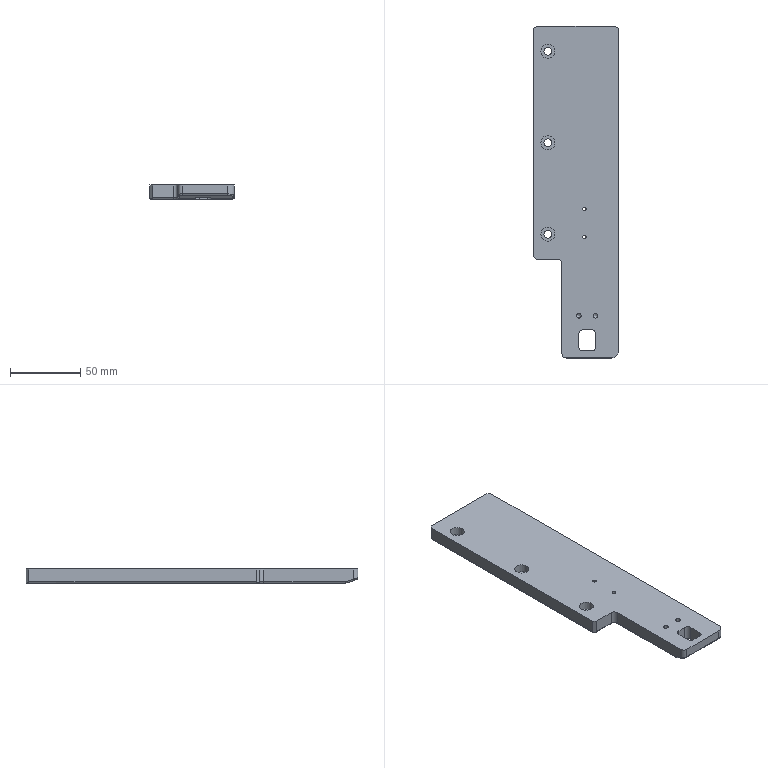NC program | NX | posted with a generic post | part box 60 x 236 x 10 mm
Lines 1177 to 2922 of 2922, first 1565 of 1740 lines:
(ZLEVEL_PROFILE_2 , TOOL : D4R0.5)
N2304 T17 M6
N2306 G54
N2308 G17 G0 G90 X-1.933 Y1.356 S9500 M3
N2310 G43 Z30. H17
N2312 Z1.488
N2314 G94 G1 Z-0.012 F3000.
N2316 X-1.63 Y0.83
N2318 G3 X-1.283 Y0.63 R0.4
N2320 G1 X0.698
N2322 X1.125 Y0.689
N2324 X164.875
N2326 G2 X166.689 Y-1.125 R1.915
N2328 G1 Y-17.
N2330 G3 X169. Y-19.311 R2.311
N2332 G1 X227.093
N2334 X227.441 Y-19.344
N2336 X229.095 Y-19.374
N2338 Y-19.313 Z-0.02
N2340 X229.094 Y-19.26 Z-0.028
N2342 X227.378 Y-19.24
N2344 X227.093 Y-19.21
N2346 X169.
N2348 G2 X166.79 Y-17. R2.21
N2350 G1 Y-1.191
N2352 G3 X164.809 Y0.79 R1.981
N2354 G1 X1.191
N2356 G2 X-1.267 Y0.741 R21.196
N2358 G1 X-1.234 Y0.83 Z-0.049
N2360 X0.863 Y0.842
N2362 X1.263 Y0.881
N2364 X164.752
N2366 G2 X166.881 Y-1.248 R2.129
N2368 G1 Y-17.
N2370 G3 X169. Y-19.119 R2.119
N2372 G1 X227.093
N2374 X227.378 Y-19.149
N2376 X229.092 Y-19.161
N2378 X229.089 Y-19.105 Z-0.063
N2380 X229.088 Y-19.063 Z-0.077
N2382 X227.232 Y-19.039
N2384 X227.093 Y-19.027
N2386 X169.
N2388 G2 X166.973 Y-17. R2.027
N2390 G1 Y-1.4
N2392 G3 X166.327 Y0.392 R2.646
N2394 X164.631 Y0.973 R2.773
N2396 G1 X1.546
N2398 G2 X-1.202 Y0.908 R23.914
N2400 G1 X-1.164 Y0.998 Z-0.11
N2402 G3 X1.546 Y1.064 R24.423
N2404 G1 X164.348
N2406 X164.631 Y1.063
N2408 X165.856 Y0.862
N2410 X166.009 Y0.8
N2412 G2 X166.917 Y-0.358 R1.468
N2414 G1 X167.064 Y-1.4
N2416 Y-17.
N2418 G3 X169. Y-18.936 R1.936
N2420 G1 X227.093
N2422 X227.254 Y-18.944
N2424 X227.378 Y-18.953
N2426 X227.661 Y-18.987
N2428 X229.087 Y-18.986
N2430 X229.086 Y-18.923 Z-0.13
N2432 Y-18.894 Z-0.15
N2434 X227.661 Y-18.896
N2436 X227.366 Y-18.863
N2438 X227.259 Y-18.858
N2440 X227.093 Y-18.847
N2442 X169.
N2444 G2 X167.153 Y-17. R1.847
N2446 G1 Y-1.681
N2448 X167.071 Y-0.473
N2450 G3 X165.738 Y1.034 R1.648
N2452 G1 X165.62 Y1.057
N2454 X164.569 Y1.15
N2456 X164.348 Y1.153
N2458 X1.546
N2460 X1.065 Y1.123
N2462 X-1.119 Y1.107
N2464 X-1.079 Y1.2 Z-0.195
N2466 G3 X1.546 Y1.24 R35.981
N2468 G1 X164.348
N2470 X165.536 Y1.173
N2472 X165.665 Y1.158
N2474 G2 X167.177 Y-0.455 R1.713
N2476 G1 X167.24 Y-1.681
N2478 Y-17.
N2480 G3 X169. Y-18.76 R1.76
N2482 G1 X227.093
N2484 G3 X229.084 Y-18.788 R19.848
N2486 G1 X229.085 Y-18.741 Z-0.221
N2488 Y-18.709 Z-0.247
N2490 X228.791 Y-18.697
N2492 X227.378 Y-18.703
N2494 X227.093 Y-18.676
N2496 X169.
N2498 G2 X167.324 Y-17. R1.676
N2500 G1 Y-1.547
N2502 X167.272 Y-0.402
N2504 G3 X165.609 Y1.264 R1.748
N2506 G1 X164.348 Y1.324
N2508 X1.547
N2510 G2 X0.774 Y1.287 R7.977
N2512 G1 X-1.035 Y1.288
N2514 X-0.987 Y1.376 Z-0.304
N2516 X1.263 Y1.381
N2518 X1.602 Y1.405
N2520 X164.398
N2522 X164.631 Y1.391
N2524 X165.657 Y1.35
N2526 G2 X167.356 Y-0.362 R1.77
N2528 G1 X167.39 Y-1.4
N2530 X167.405 Y-1.602
N2532 Y-17.
N2534 G3 X169. Y-18.595 R1.595
N2536 G1 X227.093
N2538 G3 X227.497 Y-18.618 R3.817
N2540 G1 X229.085 Y-18.628
N2542 X229.084 Y-18.592 Z-0.335
N2544 Y-18.556 Z-0.366
N2546 X227.661 Y-18.552
N2548 X227.519 Y-18.545
N2550 X227.292 Y-18.532
N2552 X227.093 Y-18.518
N2554 X169.
N2556 G2 X167.482 Y-17. R1.518
N2558 G1 Y-1.654
N2560 X167.466 Y-1.4
N2562 X167.441 Y-0.33
N2564 G3 X165.701 Y1.427 R1.799
N2566 G2 X164.346 Y1.482 R86.521
N2568 G1 X1.654
N2570 X1.546 Y1.474
N2572 X0.698 Y1.45
N2574 X-0.715 Y1.458
N2576 X-0.943 Y1.452
N2578 X-0.898 Y1.529 Z-0.434
N2580 X0.698 Y1.527
N2582 X1.546 Y1.548
N2584 X1.703 Y1.555
N2586 X164.297
N2588 X164.348 Y1.552
N2590 X165.757 Y1.504
N2592 G2 X167.518 Y-0.351 R1.825
N2594 G3 X167.555 Y-1.703 R15.073
N2596 G1 Y-17.
N2598 G3 X169. Y-18.445 R1.445
N2600 G1 X227.093
N2602 X227.286 Y-18.456
N2604 X227.481 Y-18.464
N2606 X227.661 Y-18.474
N2608 X228.509 Y-18.481
N2610 X229.083 Y-18.483
N2612 Y-18.442 Z-0.47
N2614 Y-18.412 Z-0.506
N2616 G2 X227.413 Y-18.393 R46.566
N2618 G1 X227.347 Y-18.39
N2620 X227.093 Y-18.377
N2622 X169.
N2624 G2 X167.623 Y-17. R1.377
N2626 G1 Y-1.747
N2628 G2 X167.591 Y-0.279 R21.059
N2630 G3 X165.762 Y1.577 R1.859
N2632 G2 X164.253 Y1.623 R51.61
N2634 G1 X1.747
N2636 X1.546 Y1.609
N2638 X0.698 Y1.594
N2640 X-0.715 Y1.598
N2642 X-0.85 Y1.594
N2644 X-0.798 Y1.66 Z-0.583
N2646 X-0.715 Y1.664
N2648 X0.971 Y1.66
N2650 G3 X1.791 Y1.687 R11.853
N2652 G1 X164.209
N2654 G3 X165.762 Y1.645 R86.835
N2656 G2 X167.321 Y0.842 R1.933
N2658 X167.659 Y-0.279 R1.92
N2660 G3 X167.687 Y-1.791 R14.568
N2662 G1 Y-17.
N2664 G3 X169. Y-18.313 R1.313
N2666 G1 X227.093
N2668 G3 X229.084 Y-18.34 R29.332
N2670 G1 X229.083 Y-18.306 Z-0.623
N2672 Y-18.273 Z-0.664
N2674 G2 X227.093 Y-18.255 R26.061
N2676 G1 X169.
N2678 G2 X167.745 Y-17. R1.255
N2680 G1 Y-1.828
N2682 G2 X167.72 Y-0.279 R18.813
N2684 G3 X167.406 Y0.842 R1.968
N2686 X165.762 Y1.71 R1.98
N2688 G2 X164.172 Y1.745 R28.102
N2690 G1 X1.828
N2692 G2 X1.263 Y1.718 R5.619
N2694 G1 X-0.747 Y1.721
N2696 X-0.697 Y1.774 Z-0.749
N2698 X1.263 Y1.77
N2700 G3 X1.864 Y1.798 R5.314
N2702 G1 X164.136
N2704 G3 X165.479 Y1.767 R16.419
N2706 G2 X166.234 Y1.707 R3.44
N2708 X167.773 Y-0.21 R1.898
N2710 G3 X167.798 Y-1.864 R19.045
N2712 G1 Y-17.
N2714 G3 X169. Y-18.202 R1.202
N2716 G1 X227.093
N2718 G3 X227.701 Y-18.217 R11.739
N2720 G1 X229.082
N2722 Y-18.196 Z-0.793
N2724 Y-18.172 Z-0.837
N2726 G2 X227.093 Y-18.155 R38.055
N2728 G1 X169.
N2730 G2 X167.845 Y-17. R1.155
N2732 G1 Y-1.895
N2734 G2 X167.819 Y-0.279 R20.129
N2736 G1 X167.815 Y-0.077
N2738 G3 X166.196 Y1.765 R1.895
N2740 X165.196 Y1.824 R5.764
N2742 G2 X164.105 Y1.845 R13.41
N2744 G1 X1.895
N2746 G2 X1.249 Y1.822 R8.509
N2748 G1 X-0.433 Y1.826
N2750 X-0.646 Y1.821
N2752 X-0.594 Y1.864 Z-0.928
N2754 X-0.433 Y1.866
N2756 X1.247 Y1.862
N2758 G3 X1.923 Y1.887 R8.855
N2760 G1 X164.077
N2762 G3 X165.196 Y1.864 R12.939
N2764 G2 X166.09 Y1.831 R9.187
N2766 X167.868 Y-0.096 R1.942
N2768 G1 X167.874 Y-1.681
N2770 X167.887 Y-1.923
N2772 Y-17.
N2774 G3 X169. Y-18.113 R1.113
N2776 G1 X227.093
N2778 G3 X228.691 Y-18.13 R28.373
N2780 G2 X229.081 Y-18.131 R9.816
N2782 G1 Y-18.115 Z-0.975
N2784 Y-18.096 Z-1.022
N2786 X227.988 Y-18.097
N2788 G2 X227.093 Y-18.078 R20.335
N2790 G1 X169.
N2792 G2 X167.922 Y-17. R1.078
N2794 G1 Y-1.946
N2796 X167.906 Y-1.681
N2798 X167.901 Y-0.069
N2800 G3 X166.211 Y1.851 R1.944
N2802 X165.196 Y1.901 R6.231
N2804 G2 X164.054 Y1.922 R14.096
N2806 G1 X1.946
N2808 G2 X1.378 Y1.901 R8.073
N2810 G1 X-0.433
N2812 X-0.541 Y1.898
N2814 X-0.485 Y1.927 Z-1.117
N2816 X-0.15 Y1.932
N2818 X1.263 Y1.929
N2820 G3 X1.966 Y1.95 R8.162
N2822 G1 X164.034
N2824 G3 X164.631 Y1.93 R5.549
N2826 G2 X166.035 Y1.909 R23.351
N2828 X167.934 Y-0.074 R1.988
N2830 G1 X167.937 Y-1.681
N2832 X167.95 Y-1.966
N2834 Y-17.
N2836 G3 X169. Y-18.05 R1.05
N2838 G1 X227.093
N2840 G3 X228.692 Y-18.064 R30.689
N2842 G2 X229.083 Y-18.065 R9.814
N2844 G1 X229.082 Y-18.057 Z-1.165
N2846 Y-18.043 Z-1.213
N2848 G2 X227.093 Y-18.028 R57.64
N2850 G1 X169.
N2852 G2 X167.972 Y-17. R1.028
N2854 G1 Y-1.979
N2856 X167.96 Y-1.681
N2858 X167.959 Y0.001
N2860 G3 X166.336 Y1.898 R1.982
N2862 X165.732 Y1.955 R3.456
N2864 G1 X164.255 Y1.964
N2866 X164.021 Y1.972
N2868 X1.979
N2870 G2 X1.263 Y1.957 R13.666
N2872 G1 X-0.15 Y1.959
N2874 X-0.43 Y1.956
N2876 X-0.412 Y1.973 Z-1.309
N2878 X-0.15 Y1.976
N2880 X1.546 Y1.975
N2882 X1.991 Y1.988
N2884 X164.009
N2886 X164.066 Y1.982
N2888 X165.92 Y1.972
N2890 G2 X167.175 Y1.565 R2.172
N2892 X167.976 Y0.001 R1.98
N2894 G1 Y-1.681
N2896 X167.988 Y-1.991
N2898 Y-17.
N2900 G3 X169. Y-18.012 R1.012
N2902 G1 X227.093
N2904 G3 X229.082 Y-18.023 R47.946
N2906 G1 X229.189 Y-18.015 Z-1.404
N2908 X229.117 Y-18.011
N2910 X227.378 Y-18.007
N2912 X227.093 Y-18.003
N2914 X169.
N2916 G2 X167.997 Y-17. R1.003
N2918 G1 Y-1.998
N2920 X167.991 Y-1.681
N2922 Y0.001
N2924 G3 X167.237 Y1.539 R1.985
N2926 G1 X167.233 Y1.545
N2928 X167.108 Y1.636
N2930 X167.084 Y1.648
N2932 X166.928 Y1.744
N2934 X166.86 Y1.777
N2936 X166.857 Y1.78
N2938 X166.834 Y1.79
N2940 X166.793 Y1.804
N2942 X166.786 Y1.812
N2944 X166.754 Y1.824
N2946 X166.716 Y1.838
N2948 X166.708 Y1.844
N2950 X166.53 Y1.902
N2952 X166.5 Y1.91
N2954 X166.442 Y1.924
N2956 X166.144 Y1.974
N2958 X166.044 Y1.982
N2960 X165.479 Y1.99
N2962 X164.066 Y1.994
N2964 X164.002 Y1.997
N2966 X1.998
N2968 X1.828 Y1.993
N2970 X-0.15 Y1.99
N2972 X-0.412 Y1.986
N2974 Y1.992 Z-1.5
N2976 X-0.15 Y1.998
N2978 X1.828 Y1.997
N2980 X2.111 Y2.
N2982 X165.955 Y1.997
N2984 X166.051 Y2.004
N2986 X166.145 Y1.984
N2988 G2 X166.424 Y1.934 R2.592
N2990 G1 X166.572 Y1.895
N2992 X166.61 Y1.884
N2994 X166.802 Y1.811
N2996 G2 X167.997 Y0.001 R2.
N2998 G1 X168. Y-17.
N3000 G3 X168.715 Y-17.958 R1.01
N3002 X169. Y-18. R1.
N3004 G1 X228.791 Y-18.003
N3006 X229.215 Y-18.011
N3008 G3 X229.565 Y-17.818 R0.4
N3010 G1 X229.871 Y-17.313
N3012 Z0.
N3014 G0 Z30.
N3016 X229.746 Y-61.341
N3018 Z1.488
N3020 G1 Z-0.012
N3022 X229.442 Y-60.822
N3024 G3 X229.094 Y-60.625 R0.4
N3026 G1 X227.369 Y-60.637
N3028 X227.093 Y-60.689
N3030 X1.131
N3032 X0.848 Y-60.639
N3034 X-1.781 Y-60.614
N3036 X-1.737 Y-60.71 Z-0.028
N3038 X-1.414 Y-60.707
N3040 X0.848 Y-60.74
N3042 X1.191 Y-60.79
N3044 X227.093
N3046 X229.094 Y-60.726
N3048 X229.093 Y-60.818 Z-0.039
N3050 Y-60.857 Z-0.049
N3052 X227.369 Y-60.871
N3054 X227.093 Y-60.881
N3056 X1.414
N3058 X-1.414 Y-60.827
N3060 X-1.675 Y-60.831
N3062 X-1.604 Y-60.923 Z-0.077
N3064 X1.131 Y-60.947
N3066 X1.414 Y-60.973
N3068 X227.093
N3070 X227.369 Y-60.946
N3072 X229.093 Y-60.932
N3074 Y-60.993 Z-0.093
N3076 Y-61.02 Z-0.11
N3078 X227.369 Y-61.037
N3080 X227.093 Y-61.064
N3082 X1.414
N3084 X1.131 Y-61.037
N3086 X-1.529 Y-61.014
N3088 X-1.44 Y-61.117 Z-0.15
N3090 X1.131 Y-61.144
N3092 X1.696 Y-61.153
N3094 X227.093
N3096 X229.093 Y-61.124
N3098 X229.094 Y-61.177 Z-0.172
N3100 Y-61.215 Z-0.195
N3102 X227.093 Y-61.24
N3104 X1.696
N3106 X1.131 Y-61.228
N3108 X-1.36 Y-61.21
N3110 X-1.276 Y-61.299 Z-0.247
N3112 X1.696 Y-61.324
N3114 X227.093
N3116 X227.369 Y-61.314
N3118 X229.094 Y-61.303
N3120 Y-61.345 Z-0.275
N3122 Y-61.378 Z-0.304
N3124 X227.369 Y-61.39
N3126 X227.093 Y-61.405
N3128 X1.602
N3130 X-1.183 Y-61.381
N3132 X-1.092 Y-61.461 Z-0.366
N3134 X1.654 Y-61.482
N3136 X227.093
N3138 X227.369 Y-61.468
N3140 X229.093 Y-61.452
N3142 X229.094 Y-61.492 Z-0.4
N3144 Y-61.526 Z-0.434
N3146 X227.093 Y-61.555
N3148 X1.703
N3150 X1.414 Y-61.551
N3152 X-0.566 Y-61.538
N3154 X-1.001 Y-61.535
N3156 X-0.904 Y-61.602 Z-0.506
N3158 X1.696 Y-61.617
N3160 X1.747 Y-61.623
N3162 X227.093
N3164 X227.369 Y-61.612
N3166 X229.094 Y-61.596
N3168 Y-61.632 Z-0.544
N3170 X229.093 Y-61.664 Z-0.583
N3172 X227.369 Y-61.678
N3174 X227.093 Y-61.687
N3176 X1.791
N3178 X-0.804 Y-61.671
N3180 X-0.707 Y-61.727 Z-0.664
N3182 X1.696 Y-61.737
N3184 X1.828 Y-61.745
N3186 X227.093
N3188 X227.369 Y-61.74
N3190 X228.783 Y-61.731
N3192 X229.093
N3194 Y-61.759 Z-0.706
N3196 Y-61.789 Z-0.749
N3198 X228.783 Y-61.786
N3200 X227.369 Y-61.793
N3202 X227.093 Y-61.798
N3204 X1.864
N3206 G3 X-0.608 Y-61.781 R66.741
N3208 G1 X-0.512 Y-61.83 Z-0.837
N3210 X1.696 Y-61.841
N3212 X1.895 Y-61.845
N3214 X227.093
N3216 X229.093 Y-61.833
N3218 Y-61.855 Z-0.882
N3220 X229.092 Y-61.875 Z-0.928
N3222 X228.783 Y-61.871
N3224 X227.369 Y-61.879
N3226 X227.093 Y-61.887
N3228 X1.923
N3230 X1.696 Y-61.88
N3232 X0. Y-61.871
N3234 X-0.418 Y-61.872
N3236 X-0.321 Y-61.907 Z-1.022
N3238 X1.696 Y-61.917
N3240 X1.946 Y-61.922
N3242 X227.093
N3244 X227.369 Y-61.915
N3246 X229.092 Y-61.909
N3248 X229.093 Y-61.925 Z-1.069
N3250 X229.094 Y-61.937 Z-1.117
N3252 X227.369 Y-61.941
N3254 X227.093 Y-61.95
N3256 X1.966
N3258 G3 X-0.242 Y-61.935 R91.133
N3260 G1 X-0.175 Y-61.957 Z-1.213
N3262 X1.696 Y-61.967
N3264 X1.979 Y-61.972
N3266 X227.093
N3268 X227.369 Y-61.967
N3270 X229.094 Y-61.958
N3272 X229.133 Y-61.977 Z-1.309
N3274 X227.369 Y-61.983
N3276 X227.093 Y-61.988
N3278 X1.991
N3280 X1.979 Y-61.985
N3282 X-0.137 Y-61.978
N3284 Y-61.986 Z-1.404
N3286 X0. Y-61.992
N3288 X1.998 Y-61.997
N3290 X227.093
N3292 X227.369 Y-61.994
N3294 X229.065 Y-61.992
N3296 X229.136 Y-61.99
N3298 Y-61.996 Z-1.5
N3300 X0. Y-61.997
N3302 X-0.137 Y-61.989
N3304 G3 X-0.495 Y-62.167 R0.4
N3306 G1 X-0.844 Y-62.692
N3308 Z0.
N3310 G0 Z30.
(ZLEVEL_PROFILE_2_COPY , TOOL : D4R0.5)
N3312 X222.663 Y-18.407
N3314 Z1.494
N3316 G1 Z-0.006
N3318 X222.987 Y-18.97
N3320 G3 X223.333 Y-19.171 R0.4
N3322 G1 X225.283 Y-19.175
N3324 X225.733 Y-19.249
N3326 X225.95 Y-19.316
N3328 X225.85 Y-19.357
N3330 X225.857 Y-19.366
N3332 X227.063
N3334 G2 X228.851 Y-21. R1.853
N3336 G1 Y-32.
N3338 X228.766 Y-32.5
N3340 X228.881 Y-32.501 Z-0.009
N3342 X228.896 Z-0.013
N3344 X228.967 Y-32.
N3346 Y-21.
N3348 G3 X228.201 Y-19.679 R1.61
N3350 X227.066 Y-19.305 R2.581
N3352 G1 X226.04
N3354 X226.146 Y-19.27
N3356 X225.886 Y-19.21
N3358 X225.088 Y-19.137
N3360 X224.745 Y-19.135
N3362 X223.65
N3364 X223.721 Y-19.117 Z-0.017
N3366 X223.792 Y-19.096 Z-0.021
N3368 X223.915 Y-19.1
N3370 X224.63 Y-19.099
N3372 X225.347 Y-19.113
N3374 X226.03 Y-19.173
N3376 X226.347 Y-19.224
N3378 X226.286 Y-19.251
N3380 X227.069
N3382 G2 X228.639 Y-19.936 R2.418
N3384 X229.072 Y-20.963 R1.435
N3386 G1 Y-32.
N3388 X229.03 Y-32.502
N3390 X229.092 Y-32.503 Z-0.026
N3392 X229.133 Z-0.031
N3394 X229.177 Y-32.
N3396 Y-21.
N3398 X229.011 Y-20.305
N3400 G3 X227.073 Y-19.196 R2.239
N3402 G1 X226.502
N3404 X226.549 Y-19.172
N3406 X226.502 Y-19.167
N3408 X226.08 Y-19.136
N3410 X225.849 Y-19.111
N3412 X224.485 Y-19.051
N3414 X223.93
N3416 X224.018 Y-19.024 Z-0.037
N3418 X224.106 Y-18.993 Z-0.043
N3420 X224.401 Y-18.996
N3422 X225.898 Y-19.073
N3424 X226.139 Y-19.092
N3426 X226.626 Y-19.122
N3428 X226.631 Y-19.143
N3430 X227.083
N3432 G2 X229.281 Y-21. R2.088
N3434 G1 Y-32.
N3436 X229.256 Y-32.505
N3438 X229.315 Y-32.507 Z-0.05
N3440 X229.359 Y-32.508 Z-0.057
N3442 X229.383 Y-32.
N3444 Y-21.
N3446 G3 X227.589 Y-19.149 R2.017
N3448 G1 X227.306 Y-19.112
N3450 X224.437 Y-18.933
N3452 X224.384 Y-18.932
N3454 X224.325
N3456 X224.446 Y-18.914 Z-0.061
N3458 X224.568 Y-18.905 Z-0.065
N3460 X224.69 Y-18.899 Z-0.069
N3462 X224.811 Y-18.894 Z-0.073
N3464 G2 X227.589 Y-19.103 R86.326
N3466 X229.485 Y-21. R2.068
N3468 G1 Y-32.
N3470 X229.465 Y-32.51
N3472 X229.527 Y-32.512 Z-0.082
N3474 X229.578 Y-32.514 Z-0.09
N3476 X229.586 Y-32.
N3478 Y-21.
N3480 G3 X229.312 Y-20.102 R1.84
N3482 X227.704 Y-19.067 R2.221
N3484 G1 X227.306 Y-19.016
N3486 G2 X225.18 Y-18.873 R49.946
N3488 G1 X225.3 Y-18.864 Z-0.097
N3490 X225.42 Y-18.857 Z-0.103
N3492 X225.539 Y-18.853 Z-0.11
N3494 G2 X227.872 Y-19.053 R19.708
N3496 X229.686 Y-21. R2.124
N3498 G1 Y-32.002
N3500 X229.671 Y-32.521
N3502 X229.732 Y-32.526 Z-0.12
N3504 X229.772 Y-32.529 Z-0.131
N3506 X229.786 Y-32.006
N3508 Y-21.
N3510 G3 X227.819 Y-18.963 R2.254
N3512 G1 X227.306 Y-18.9
N3514 X225.84 Y-18.829
N3516 X225.96 Y-18.823 Z-0.139
N3518 X226.08 Y-18.817 Z-0.146
N3520 X226.201 Y-18.81 Z-0.154
N3522 X227.698 Y-18.892
N3524 X228.119 Y-18.982
N3526 G2 X229.885 Y-21. R2.238
N3528 G1 Y-32.012
N3530 X229.875 Y-32.539
N3532 X229.929 Y-32.548 Z-0.166
N3534 X229.969 Y-32.554 Z-0.179
N3536 X229.983 Y-32.023
N3538 Y-21.
N3540 G3 X228.437 Y-19.022 R2.241
N3542 X226.459 Y-18.79 R5.673
N3544 G1 X226.529 Y-18.766 Z-0.192
N3546 X226.6 Y-18.738 Z-0.205
N3548 G2 X228.719 Y-19.078 R5.009
N3550 X230.081 Y-21. R2.214
N3552 G1 Y-32.034
N3554 X230.069 Y-32.57
N3556 X230.124 Y-32.581 Z-0.219
N3558 X230.168 Y-32.589 Z-0.233
N3560 X230.178 Y-32.049
N3562 Y-21.
N3564 G3 X228.719 Y-19.012 R2.279
N3566 X226.459 Y-18.697 R5.595
N3568 G1 Y-18.651 Z-0.263
N3570 G2 X228.719 Y-18.956 R5.798
N3572 X230.274 Y-21. R2.298
N3574 G1 Y-32.066
N3576 X230.266 Y-32.173
N3578 X230.261 Y-32.611
N3580 X230.317 Y-32.625 Z-0.279
N3582 X230.359 Y-32.635 Z-0.295
N3584 X230.37 Y-32.086
N3586 Y-21.
N3588 G3 X229.002 Y-19.014 R2.3
N3590 X226.741 Y-18.607 R5.136
N3592 G1 X226.859 Y-18.594 Z-0.306
N3594 X226.976 Y-18.579 Z-0.317
N3596 X227.093 Y-18.564 Z-0.328
N3598 G2 X229.002 Y-18.954 R4.904
N3600 X230.464 Y-21. R2.34
N3602 G1 Y-32.108
N3604 X230.457 Y-32.663
N3606 X230.55 Y-32.696 Z-0.362
N3608 X230.555 Y-32.132
N3610 Y-21.
N3612 G3 X229.001 Y-18.892 R2.414
N3614 X226.741 Y-18.523 R5.534
N3616 G1 Y-18.484 Z-0.396
N3618 G2 X229.127 Y-18.892 R5.537
N3620 X230.647 Y-21. R2.395
N3622 G1 Y-32.163
N3624 X230.646 Y-32.73
N3626 X230.738 Y-32.774 Z-0.431
N3628 X230.74 Y-32.198
N3630 Y-21.
N3632 G3 X230.299 Y-19.728 R2.052
N3634 X228.719 Y-18.688 R3.007
N3636 X226.741 Y-18.448 R6.256
N3638 G1 Y-18.413 Z-0.466
N3640 G2 X228.602 Y-18.61 R6.886
N3642 X230.161 Y-19.457 R3.32
N3644 X230.834 Y-21. R2.208
N3646 G1 Y-32.233
N3648 Y-32.738
N3650 X230.83 Y-32.824
N3652 X230.924 Y-32.874 Z-0.501
N3654 X230.928 Y-32.276
N3656 Y-21.
N3658 G3 X230.254 Y-19.457 R2.207
N3660 X228.437 Y-18.527 R3.604
N3662 X226.741 Y-18.381 R7.874
N3664 G1 Y-18.35 Z-0.536
N3666 G2 X228.437 Y-18.488 R8.885
N3668 X230.132 Y-19.265 R3.873
N3670 G1 X230.323 Y-19.436
N3672 G2 X231.021 Y-20.999 R2.099
N3674 G1 Y-32.32
N3676 X231.019 Y-32.93
N3678 X231.114 Y-32.992 Z-0.572
N3680 X231.115 Y-32.37
N3682 Y-21.
N3684 G3 X230.441 Y-19.457 R2.204
N3686 X228.719 Y-18.521 R3.701
N3688 X226.87 Y-18.322 R7.598
N3690 G1 X226.764 Y-18.295 Z-0.607
N3692 G2 X228.437 Y-18.425 R8.878
N3694 X230.219 Y-19.175 R4.294
N3696 X231.209 Y-21. R2.342
N3698 G1 Y-32.423
N3700 X231.206 Y-33.061
N3702 X231.298 Y-33.14 Z-0.642
N3704 X231.302 Y-32.482
N3706 Y-21.
N3708 G3 X230.313 Y-19.175 R2.343
N3710 X228.437 Y-18.396 R4.362
N3712 X226.594 Y-18.27 R10.185
N3714 G1 X226.592 Y-18.246 Z-0.677
N3716 G2 X228.154 Y-18.318 R12.163
N3718 X230.406 Y-19.175 R4.894
N3720 X231.396 Y-21. R2.344
N3722 G1 Y-32.544
N3724 X231.393 Y-33.226
N3726 X231.489 Y-33.313 Z-0.712
N3728 Y-32.613
N3730 Y-21.
N3732 G3 X230.5 Y-19.175 R2.345
N3734 X227.872 Y-18.261 R5.289
N3736 X226.59 Y-18.224 R17.368
N3738 G1 X226.589 Y-18.203 Z-0.747
N3740 G2 X228.154 Y-18.265 R14.643
N3742 X230.594 Y-19.175 R5.339
N3744 X231.583 Y-21. R2.346
N3746 G1 Y-32.687
N3748 X231.579 Y-33.421
N3750 X231.63 Y-33.479 Z-0.765
N3752 X231.675 Y-33.537 Z-0.782
N3754 X231.677 Y-32.768
N3756 Y-21.
N3758 G3 X230.687 Y-19.175 R2.347
N3760 X228.154 Y-18.244 R5.373
N3762 X226.588 Y-18.183 R14.486
N3764 G1 X226.589 Y-18.164 Z-0.817
N3766 G2 X228.437 Y-18.261 R12.887
N3768 X230.781 Y-19.175 R5.416
N3770 X231.77 Y-21. R2.351
N3772 G1 Y-33.586
N3774 X231.766 Y-33.669
N3776 X231.817 Y-33.746 Z-0.835
N3778 X231.863 Y-33.823 Z-0.853
N3780 X231.864 Y-32.951
N3782 Y-21.
N3784 G3 X230.875 Y-19.175 R2.349
N3786 X228.437 Y-18.241 R5.533
N3788 X226.59 Y-18.147 R13.251
N3790 G1 X226.592 Y-18.131 Z-0.888
N3792 G2 X228.437 Y-18.222 R13.563
N3794 X230.968 Y-19.175 R5.656
N3796 X231.958 Y-21. R2.35
N3798 G1 Y-33.868
N3800 X231.952 Y-34.022
N3802 X232.004 Y-34.145 Z-0.905
N3804 X232.044 Y-34.267 Z-0.923
N3806 X232.051 Y-34.151
N3808 Y-21.
N3810 G3 X231.062 Y-19.175 R2.354
N3812 X228.719 Y-18.244 R5.823
N3814 X226.583 Y-18.116 R12.291
N3816 G2 X226.231 Y-17.925 R0.4
N3818 G1 X225.857 Y-17.316
N3820 Z0.577
N3822 G0 Z30.
N3824 X229.46 Y-42.791
N3826 Z1.494
N3828 G1 Z-0.006
N3830 X228.834 Y-43.312
N3832 G3 X228.765 Y-43.5 R0.2
N3834 G1 X228.851 Y-44.
N3836 Y-58.956
N3838 G2 X227.677 Y-60.441 R1.526
N3840 G1 X226.86 Y-60.634
N3842 X226.341
N3844 X226.399 Y-60.675
N3846 X226.343 Y-60.687
N3848 X225.842 Y-60.748
N3850 G2 X224.763 Y-60.83 R11.791
N3852 G3 X224.172 Y-60.831 R1.81
N3854 X223.863 Y-61.085 R0.4
N3856 G1 X223.661 Y-61.623
N3858 Z1.494
N3860 G0 X223.748 Y-61.669 Z1.487
N3862 G1 Z-0.013
N3864 X224.136 Y-61.051
N3866 G2 X224.489 Y-60.864 R0.4
N3868 G3 X225.911 Y-60.787 R7.818
N3870 G1 X226.356 Y-60.73
N3872 X226.391 Y-60.695
N3874 X226.852
N3876 X227.589 Y-60.573
N3878 G3 X228.967 Y-59. R1.694
N3880 G1 Y-44.
N3882 X228.9 Y-43.499
N3884 X228.99 Z-0.017
N3886 X229.033 Y-43.498 Z-0.021
N3888 X229.072 Y-44.
N3890 Y-59.
N3892 G2 X227.808 Y-60.598 R1.8
N3894 G1 X227.436 Y-60.713
N3896 X226.741 Y-60.749
N3898 X226.379
N3900 X226.396 Y-60.779
N3902 X226.052 Y-60.822
N3904 X225.867 Y-60.843
N3906 X225.435 Y-60.886
N3908 X225.328 Y-60.897
N3910 X224.631 Y-60.906
N3912 X224.728 Y-60.931 Z-0.026
N3914 X224.825 Y-60.955 Z-0.031
N3916 X224.905
N3918 X225.328 Y-60.949
N3920 X225.385 Y-60.944
N3922 X226.515 Y-60.831
N3924 X226.511 Y-60.804
N3926 X226.741
N3928 X227.419 Y-60.749
N3930 G3 X229.177 Y-59. R1.918
N3932 G1 Y-44.
N3934 X229.137 Y-43.497
N3936 X229.206 Y-43.495 Z-0.037
N3938 X229.261 Y-43.494 Z-0.043
N3940 X229.281 Y-44.
N3942 Y-59.
N3944 G2 X227.872 Y-60.732 R1.971
N3946 G1 X227.341 Y-60.824
N3948 G2 X226.741 Y-60.857 R2.58
N3950 G3 X226.383 Y-61.035 R0.4
N3952 G1 X225.9 Y-61.764
N3954 Z1.457
N3956 G0 X224.754 Y-61.898 Z1.443
N3958 G1 Z-0.057
N3960 X225.021 Y-61.311
N3962 G2 X225.347 Y-61.079 R0.4
N3964 G1 X227.306 Y-60.89
N3966 X227.812 Y-60.79
N3968 G3 X229.383 Y-59. R1.955
N3970 G1 Y-44.
N3972 X229.362 Y-43.492
N3974 X229.414 Y-43.491 Z-0.065
N3976 X229.467 Y-43.49 Z-0.073
N3978 X229.485 Y-44.
N3980 Y-59.
N3982 G2 X227.669 Y-60.884 R2.048
N3984 G1 X225.894 Y-61.082
N3986 X225.634 Y-61.116
N3988 X225.736 Y-61.129 Z-0.082
N3990 X225.837 Y-61.138 Z-0.09
N3992 X226.537 Y-61.038
N3994 X226.654 Y-61.03
N3996 X226.702 Y-61.013
N3998 X226.865
N4000 X227.024 Y-61.01
N4002 X227.796 Y-60.908
N4004 G3 X229.586 Y-59. R2.067
N4006 G1 Y-44.
N4008 X229.58 Y-43.486
N4010 X229.632 Y-43.483 Z-0.1
N4012 X229.679 Y-43.48 Z-0.11
N4014 X229.686 Y-43.998
N4016 Y-59.
N4018 G2 X228.426 Y-60.776 R2.06
N4020 X226.884 Y-61.063 R3.714
N4022 G1 X226.627
N4024 X226.549 Y-61.082
N4026 X226.539 Y-61.077
N4028 X226.176 Y-61.128
N4030 X226.271 Y-61.133 Z-0.117
N4032 X226.365 Y-61.134 Z-0.124
N4034 X226.459 Y-61.131 Z-0.131
N4036 X226.541 Y-61.12
N4038 X226.551 Y-61.113
N4040 X226.914
N4042 G3 X228.294 Y-60.904 R4.359
N4044 X229.786 Y-59. R2.158
N4046 G1 Y-43.994
N4048 X229.782 Y-43.473
N4050 X229.833 Y-43.466 Z-0.142
N4052 X229.878 Y-43.461 Z-0.154
N4054 X229.885 Y-43.988
N4056 Y-59.
N4058 G2 X228.586 Y-60.842 R2.145
N4060 X226.923 Y-61.162 R3.999
N4062 G1 X226.554
N4064 X226.459 Y-61.178
N4066 X226.592 Z-0.162
N4068 X226.727 Y-61.193 Z-0.17
N4070 X226.861 Y-61.21 Z-0.179
N4072 G3 X228.858 Y-60.766 R3.881
N4074 X229.983 Y-59. R2.115
N4076 G1 Y-43.977
N4078 X229.97 Y-43.446
N4080 X230.028 Y-43.437 Z-0.192
N4082 X230.07 Y-43.43 Z-0.205
N4084 X230.081 Y-43.966
N4086 Y-59.
N4088 G2 X228.719 Y-60.91 R2.179
N4090 X226.589 Y-61.257 R4.616
N4092 G1 X226.6 Y-61.308 Z-0.233
N4094 G3 X228.719 Y-60.988 R5.533
N4096 X230.178 Y-59. R2.263
N4098 G1 Y-43.951
N4100 X230.168 Y-43.411
N4102 X230.222 Y-43.398 Z-0.248
N4104 X230.26 Y-43.389 Z-0.263
N4106 X230.274 Y-43.934
N4108 Y-59.
N4110 G2 X229.002 Y-60.918 R2.251
N4112 X226.84 Y-61.349 R4.721
N4114 G1 X226.913 Y-61.393 Z-0.295
N4116 X227.024 Y-61.39
N4118 X227.661 Y-61.339
N4120 G3 X229.162 Y-60.901 R3.879
N4122 X230.37 Y-59. R2.272
N4124 G1 Y-43.914
N4126 X230.358 Y-43.365
N4128 X230.455 Y-43.336 Z-0.328
N4130 X230.464 Y-43.892
N4132 Y-59.
N4134 G2 X229.285 Y-60.903 R2.29
N4136 X227.589 Y-61.392 R3.992
N4138 G1 X226.96 Y-61.436
N4140 X226.966 Y-61.477 Z-0.362
N4142 X227.772 Y-61.412
N4144 G3 X229.47 Y-60.858 R3.848
N4146 X230.555 Y-59. R2.272
N4148 G1 Y-43.868
N4150 X230.548 Y-43.302
N4152 X230.644 Y-43.268 Z-0.396
N4154 X230.647 Y-43.837
N4156 Y-59.
N4158 G2 X229.757 Y-60.732 R2.271
N4160 X228.413 Y-61.349 R3.349
N4162 X226.946 Y-61.516 R7.796
N4164 G1 X226.924 Y-61.552 Z-0.431
N4166 G3 X227.992 Y-61.469 R6.288
N4168 G1 X228.154 Y-61.442
N4170 G3 X229.567 Y-60.934 R3.777
N4172 X230.74 Y-59. R2.322
N4174 G1 Y-43.802
N4176 Y-43.228
N4178 X230.833 Y-43.18 Z-0.466
N4180 X230.834 Y-43.767
N4182 Y-59.
N4184 G2 X230.456 Y-60.18 R2.03
N4186 X228.804 Y-61.329 R2.99
N4188 G1 X228.719 Y-61.352
N4190 G2 X226.902 Y-61.587 R6.023
N4192 G1 X226.925 Y-61.619 Z-0.501
N4194 G3 X228.154 Y-61.528 R7.188
N4196 X229.992 Y-60.777 R4.172
N4198 X230.928 Y-59. R2.272
N4200 G1 Y-43.724
N4202 X230.924 Y-43.127
N4204 X231.018 Y-43.068 Z-0.536
N4206 X231.021 Y-43.68
N4208 Y-59.
N4210 G2 X229.914 Y-60.906 R2.397
N4212 X228.154 Y-61.567 R4.609
N4214 G1 X227.872 Y-61.599
N4216 G2 X226.936 Y-61.65 R9.242
N4218 G1 X226.901 Y-61.678 Z-0.572
N4220 G3 X228.368 Y-61.56 R8.663
N4222 X230.266 Y-60.713 R4.141
N4224 X231.115 Y-59. R2.302
N4226 G1 Y-43.63
N4228 X231.112 Y-43.002
N4230 X231.207 Y-42.936 Z-0.607
N4232 X231.209 Y-43.577
N4234 Y-59.
N4236 G2 X230.36 Y-60.713 R2.302
N4238 X228.437 Y-61.577 R4.259
N4240 X226.576 Y-61.705 R9.602
N4242 G1 X226.586 Y-61.73 Z-0.642
N4244 G3 X228.437 Y-61.605 R10.22
N4246 X230.453 Y-60.713 R4.329
N4248 X231.302 Y-59. R2.302
N4250 G1 Y-43.518
N4252 X231.299 Y-42.859
N4254 X231.391 Y-42.769 Z-0.677
N4256 X231.396 Y-43.456
N4258 Y-59.
N4260 G2 X230.303 Y-60.897 R2.453
N4262 X228.154 Y-61.682 R4.903
N4264 X226.59 Y-61.754 R12.231
N4266 G1 X226.581 Y-61.776 Z-0.712
N4268 G3 X228.154 Y-61.708 R13.798
N4270 X230.573 Y-60.763 R4.957
N4272 X231.489 Y-59. R2.265
N4274 G1 Y-43.387
N4276 X231.486 Y-42.68
N4278 X231.58 Y-42.578 Z-0.747
N4280 X231.583 Y-43.313
N4282 Y-59.
N4284 G2 X230.461 Y-60.919 R2.432
N4286 X227.872 Y-61.759 R5.438
N4288 X226.587 Y-61.797 R16.32
N4290 G1 X226.581 Y-61.817 Z-0.782
N4292 G3 X228.719 Y-61.664 R10.671
N4294 X230.828 Y-60.713 R4.911
N4296 X231.677 Y-59. R2.301
N4298 G1 Y-43.232
N4300 X231.672 Y-42.456
N4302 X231.724 Y-42.394 Z-0.8
N4304 X231.769 Y-42.332 Z-0.817
N4306 X231.77 Y-43.146
N4308 Y-59.
N4310 G2 X230.863 Y-60.756 R2.253
N4312 X228.437 Y-61.733 R5.139
N4314 X226.576 Y-61.836 R11.851
N4316 G1 X226.459 Y-61.853 Z-0.853
N4318 G3 X228.358 Y-61.767 R14.061
N4320 X230.757 Y-60.909 R5.572
N4322 X231.864 Y-59. R2.432
N4324 G1 Y-43.049
N4326 X231.861 Y-42.174
N4328 X231.911 Y-42.078 Z-0.87
N4330 X231.952 Y-41.981 Z-0.888
N4332 X231.958 Y-42.063
N4334 Y-59.
N4336 G2 X231.047 Y-60.759 R2.273
N4338 X229.036 Y-61.668 R5.107
N4340 X227.304 Y-61.859 R8.982
N4342 G1 X226.459 Y-61.869
N4344 Y-61.884 Z-0.923
N4346 X227.306 Y-61.875
N4348 G3 X229.42 Y-61.593 R8.041
N4350 X231.122 Y-60.773 R5.179
N4352 X232.051 Y-59. R2.275
N4354 G1 Y-42.828
N4356 X232.048 Y-41.742
N4358 G2 X232.247 Y-41.395 R0.4
N4360 G1 X232.777 Y-41.086
N4362 Z0.577
N4364 G0 X225.871 Y-17.301 Z0.542
N4366 G1 Z-0.958
N4368 X226.236 Y-17.908
N4370 G3 X226.586 Y-18.101 R0.4
N4372 G2 X228.154 Y-18.154 R15.19
N4374 X230.415 Y-18.738 R6.986
N4376 X231.685 Y-19.702 R3.364
N4378 X232.145 Y-20.997 R2.054
N4380 G1 Y-33.3
N4382 X232.144 Y-34.674
N4384 X232.138 Y-35.281
N4386 X232.143 Y-41.315
N4388 X232.145 Y-42.7
N4390 Y-59.
N4392 G2 X231.216 Y-60.772 R2.273
N4394 X229.517 Y-61.595 R5.229
N4396 X227.425 Y-61.889 R8.165
N4398 G1 X226.459 Y-61.899
N4400 Y-61.912 Z-0.993
N4402 X227.589 Y-61.899
N4404 G3 X229.914 Y-61.5 R8.194
N4406 X231.33 Y-60.759 R4.794
N4408 X232.239 Y-59. R2.302
N4410 G1 Y-21.
N4412 G3 X230.898 Y-18.935 R2.526
N4414 X228.154 Y-18.137 R7.09
N4416 X226.59 Y-18.088 R18.24
N4418 G1 X226.582 Y-18.076 Z-1.028
N4420 G2 X227.872 Y-18.102 R33.588
N4422 X230.698 Y-18.785 R7.55
N4424 X232.033 Y-19.938 R3.086
N4426 X232.332 Y-20.963 R1.904
N4428 G1 Y-59.
N4430 G2 X231.425 Y-60.757 R2.275
N4432 X229.814 Y-61.56 R4.864
N4434 G1 X229.567 Y-61.628
N4436 G2 X227.872 Y-61.898 R7.843
N4438 X226.459 Y-61.924 R24.859
N4440 G1 Y-61.935 Z-1.063
N4442 G3 X227.589 Y-61.922 R36.047
N4444 X230.099 Y-61.5 R8.588
N4446 X231.512 Y-60.763 R4.831
N4448 X232.426 Y-59. R2.302
N4450 G1 Y-20.959
N4452 G3 X232.124 Y-19.935 R1.888
N4454 X230.698 Y-18.739 R3.151
N4456 X227.872 Y-18.091 R7.859
N4458 X226.587 Y-18.065 R31.743
N4460 G1 X226.727 Z-1.068
N4462 X226.867 Y-18.064 Z-1.073
N4464 X227.008 Y-18.062 Z-1.078
N4466 X227.148 Z-1.083
N4468 X227.288 Y-18.063 Z-1.088
N4470 X227.428 Y-18.064 Z-1.093
N4472 X227.568 Y-18.069 Z-1.098
N4474 G2 X228.154 Y-18.097 R23.753
N4476 X230.98 Y-18.834 R7.737
N4478 G1 X231.094 Y-18.892
N4480 X231.455 Y-19.126
N4482 G2 X232.519 Y-21. R2.338
N4484 G1 Y-59.
N4486 G2 X231.67 Y-60.713 R2.302
N4488 X230.415 Y-61.419 R4.44
N4490 X227.872 Y-61.921 R8.353
N4492 X227.498 Y-61.934 R28.942
N4494 G1 X227.609 Y-61.935 Z-1.11
N4496 X227.72 Y-61.934 Z-1.122
N4498 X227.83 Y-61.933 Z-1.133
N4500 X227.872 Y-61.931
N4502 G3 X230.295 Y-61.497 R8.874
N4504 X231.701 Y-60.762 R4.814
N4506 X232.613 Y-59. R2.302
N4508 G1 Y-20.963
N4510 G3 X232.314 Y-19.938 R1.903
N4512 X230.98 Y-18.785 R3.086
N4514 X228.154 Y-18.086 R8.022
N4516 X227.865 Y-18.07 R21.129
N4518 G1 X227.99 Y-18.069 Z-1.151
N4520 X228.115 Y-18.073 Z-1.169
N4522 X228.154 Y-18.075
N4524 G2 X230.98 Y-18.74 R8.281
N4526 X232.405 Y-19.935 R3.152
N4528 X232.707 Y-20.959 R1.887
N4530 G1 Y-59.
N4532 G2 X231.817 Y-60.744 R2.303
N4534 X230.607 Y-61.415 R4.509
N4536 X228.154 Y-61.925 R8.557
N4538 G1 X228.044 Y-61.931
N4540 X228.166 Y-61.939 Z-1.204
N4542 G3 X230.66 Y-61.432 R9.085
N4544 X231.951 Y-60.713 R4.433
N4546 X232.8 Y-59. R2.308
N4548 G1 Y-21.
N4550 G3 X232.12 Y-19.457 R2.182
N4552 X230.769 Y-18.61 R3.689
N4554 X228.248 Y-18.066 R9.095
N4556 G1 X228.332 Y-18.071 Z-1.221
N4558 X228.417 Y-18.069 Z-1.239
N4560 G2 X230.862 Y-18.61 R9.273
N4562 X232.214 Y-19.457 R3.673
N4564 G1 X232.398 Y-19.669
N4566 G2 X232.894 Y-20.997 R2.024
N4568 G1 Y-59.
N4570 G2 X232.044 Y-60.713 R2.313
N4572 X230.375 Y-61.56 R4.861
N4574 X228.418 Y-61.93 R9.765
N4576 G1 X228.491 Y-61.926 Z-1.256
N4578 X228.565 Y-61.927 Z-1.274
N4580 G3 X230.698 Y-61.482 R9.539
N4582 X232.138 Y-60.713 R4.459
N4584 X232.988 Y-59. R2.306
N4586 G1 Y-21.
N4588 G3 X232.303 Y-19.453 R2.182
N4590 X230.833 Y-18.563 R4.092
N4592 X228.521 Y-18.067 R9.738
N4594 G1 X228.634 Y-18.077 Z-1.291
N4596 X228.748 Y-18.08 Z-1.309
N4598 G2 X230.826 Y-18.525 R10.273
N4600 X232.387 Y-19.444 R4.188
N4602 X233.081 Y-21. R2.183
N4604 G1 Y-59.001
N4606 G2 X232.555 Y-60.375 R2.057
N4608 X230.98 Y-61.418 R3.751
N4610 X228.708 Y-61.924 R9.668
N4612 G1 X228.81 Y-61.923 Z-1.344
N4614 G3 X230.836 Y-61.505 R10.019
N4616 X232.367 Y-60.664 R4.493
N4618 X233.175 Y-58.997 R2.264
N4620 G1 Y-20.996
N4622 G3 X232.681 Y-19.672 R2.023
N4624 G1 X232.495 Y-19.457
N4626 G3 X231.143 Y-18.61 R3.674
N4628 X228.768 Y-18.07 R9.614
N4630 G1 X228.849 Y-18.078 Z-1.362
N4632 X228.93 Z-1.379
N4634 G2 X231.237 Y-18.61 R9.588
N4636 X232.589 Y-19.457 R3.652
N4638 G1 X232.775 Y-19.672
N4640 G2 X233.269 Y-20.996 R2.022
N4642 G1 Y-58.992
N4644 G2 X232.393 Y-60.73 R2.344
N4646 X230.75 Y-61.56 R4.766
N4648 X228.929 Y-61.921 R10.185
N4650 G1 X228.993 Y-61.926 Z-1.414
N4652 G3 X231.263 Y-61.417 R9.761
N4654 X232.676 Y-60.536 R3.674
N4656 G1 X232.778 Y-60.43
N4658 G3 X233.362 Y-58.986 R2.202
N4660 G1 Y-21.
N4662 G3 X232.682 Y-19.457 R2.184
N4664 X231.331 Y-18.61 R3.689
N4666 X229.02 Y-18.077 R9.583
N4668 G1 X229.086 Y-18.074 Z-1.449
N4670 G2 X231.424 Y-18.61 R9.636
N4672 X232.776 Y-19.457 R3.674
N4674 G1 X232.963 Y-19.674
N4676 G2 X233.456 Y-20.996 R2.021
N4678 G1 Y-58.976
N4680 G2 X232.512 Y-60.773 R2.427
N4682 X230.937 Y-61.56 R4.615
N4684 X229.113 Y-61.921 R10.504
N4686 G1 X229.194 Y-61.923 Z-1.485
N4688 G3 X231.031 Y-61.56 R10.547
N4690 X232.684 Y-60.713 R4.612
N4692 X233.549 Y-58.966 R2.408
N4694 G1 Y-21.
N4696 G3 X232.87 Y-19.458 R2.185
N4698 X231.406 Y-18.567 R4.05
N4700 X229.168 Y-18.073 R9.877
N4702 G1 X229.296 Y-18.079 Z-1.52
N4704 G2 X230.727 Y-18.327 R12.181
N4706 X232.654 Y-19.175 R5.725
N4708 X233.643 Y-21. R2.358
N4710 G1 Y-58.952
N4712 G2 X232.763 Y-60.713 R2.442
N4714 X231.284 Y-61.513 R4.303
N4716 X229.207 Y-61.932 R10.655
N4718 G1 X229.327 Y-61.92 Z-1.537
N4720 X229.447 Y-61.911 Z-1.555
N4722 X229.567 Y-61.896
N4724 X229.806 Y-61.866
N4726 G3 X231.838 Y-61.335 R8.028
N4728 X232.676 Y-60.847 R3.46
N4730 G1 X232.853 Y-60.713
N4732 G3 X233.737 Y-58.937 R2.455
N4734 G1 Y-21.
N4736 G3 X232.747 Y-19.175 R2.359
N4738 X231.299 Y-18.465 R4.968
N4740 X229.413 Y-18.081 R10.54
N4742 G1 X229.497 Y-18.083 Z-1.59
N4744 G2 X230.914 Y-18.327 R12.499
N4746 X232.841 Y-19.175 R5.694
N4748 X233.83 Y-21. R2.359
N4750 G1 Y-58.918
N4752 G2 X232.937 Y-60.713 R2.492
N4754 X231.312 Y-61.56 R4.395
N4756 X229.417 Y-61.93 R11.202
N4758 G1 X229.505 Y-61.921 Z-1.607
N4760 X229.594 Y-61.919 Z-1.625
N4762 G3 X231.251 Y-61.61 R11.993
N4764 X233.011 Y-60.716 R4.616
N4766 X233.924 Y-58.898 R2.495
N4768 G1 Y-21.
N4770 G3 X232.934 Y-19.175 R2.359
N4772 X231.008 Y-18.327 R5.728
N4774 X229.587 Y-18.081 R12.12
N4776 G1 X229.681 Y-18.082 Z-1.66
N4778 G2 X231.146 Y-18.338 R12.457
N4780 X233.028 Y-19.175 R5.563
N4782 X234.018 Y-21. R2.359
N4784 G1 Y-58.875
N4786 G2 X233.38 Y-60.43 R2.458
N4788 X231.849 Y-61.441 R3.881
N4790 X230.047 Y-61.871 R8.406
N4792 G1 X229.85 Y-61.895
N4794 G2 X229.646 Y-61.921 R11.834
N4796 G1 X229.766 Y-61.922 Z-1.695
N4798 G3 X231.455 Y-61.602 R11.521
N4800 X233.253 Y-60.637 R4.47
N4802 X234.111 Y-58.85 R2.542
N4804 G1 Y-21.
N4806 G3 X233.112 Y-19.168 R2.359
N4808 X231.68 Y-18.468 R5.039
N4810 X229.765 Y-18.078 R10.326
N4812 G1 X229.851 Y-18.076 Z-1.73
N4814 G2 X231.982 Y-18.536 R10.112
N4816 X233.514 Y-19.447 R4.155
N4818 X234.205 Y-21. R2.185
N4820 G1 Y-58.823
N4822 G2 X233.309 Y-60.658 R2.662
N4824 X231.484 Y-61.623 R4.409
N4826 X229.852 Y-61.922 R12.049
N4828 G1 X229.95 Y-61.917 Z-1.765
N4830 X230.132 Y-61.895
N4832 X230.339 Y-61.869
N4834 G3 X232.006 Y-61.48 R8.072
N4836 X233.597 Y-60.447 R3.989
N4838 X234.298 Y-58.792 R2.593
N4840 G1 Y-21.
N4842 G3 X233.309 Y-19.175 R2.357
N4844 X231.858 Y-18.465 R4.966
N4846 X229.926 Y-18.075 R10.612
N4848 G1 X230.031 Y-18.074 Z-1.801
N4850 G2 X231.937 Y-18.461 R10.763
N4852 X233.397 Y-19.171 R5.027
N4854 X234.392 Y-21. R2.357
N4856 G1 Y-58.76
N4858 G2 X233.475 Y-60.638 R2.778
N4860 X231.517 Y-61.663 R4.497
N4862 X230.06 Y-61.919 R12.214
N4864 G1 X230.093 Y-61.926 Z-1.836
N4866 G3 X231.545 Y-61.677 R11.98
N4868 X233.757 Y-60.43 R4.466
N4870 X234.486 Y-58.723 R2.674
N4872 G1 Y-21.
N4874 G3 X233.799 Y-19.451 R2.182
N4876 X232.241 Y-18.528 R4.148
N4878 X230.104 Y-18.069 R10.638
N4880 G1 X230.223 Y-18.079 Z-1.871
N4882 G2 X231.663 Y-18.327 R12.413
N4884 X233.59 Y-19.175 R5.563
N4886 X234.579 Y-21. R2.355
N4888 G1 Y-58.686
N4890 G2 X233.806 Y-60.45 R2.703
N4892 X231.545 Y-61.702 R4.613
N4894 X230.255 Y-61.917 R12.537
N4896 G1 X230.29 Y-61.925 Z-1.906
N4898 G3 X231.545 Y-61.72 R12.173
N4900 X233.89 Y-60.43 R4.578
N4902 X234.673 Y-58.645 R2.75
N4904 G1 Y-21.
N4906 G3 X233.679 Y-19.172 R2.355
N4908 X232.218 Y-18.461 R5.031
N4910 X230.309 Y-18.074 R10.756
N4912 G1 X230.366 Y-18.067 Z-1.941
N4914 G2 X232.524 Y-18.529 R10.623
N4916 X234.081 Y-19.452 R4.148
N4918 X234.767 Y-21. R2.18
N4920 G1 Y-58.601
N4922 G2 X234.001 Y-60.38 R2.883
N4924 X232.182 Y-61.56 R4.44
N4926 X230.961 Y-61.852 R7.092
N4928 X230.426 Y-61.92 R13.63
N4930 G1 X230.483 Y-61.921 Z-1.976
N4932 G3 X230.698 Y-61.894 R11.808
N4934 G1 X230.945 Y-61.864
N4936 G3 X232.257 Y-61.56 R6.387
N4938 X234.125 Y-60.315 R4.457
N4940 X234.86 Y-58.555 R2.921
N4942 G1 Y-21.
N4944 G3 X233.871 Y-19.175 R2.353
N4946 X231.944 Y-18.327 R5.563
N4948 X230.525 Y-18.082 R12.43
N4950 G1 X230.569 Y-18.071 Z-2.011
N4952 G2 X232.512 Y-18.465 R10.75
N4954 X233.96 Y-19.172 R4.989
N4956 X234.954 Y-21. R2.36
N4958 G1 Y-58.505
N4960 G2 X234.371 Y-60.092 R2.792
N4962 X232.329 Y-61.561 R4.428
N4964 X231.012 Y-61.867 R6.347
N4966 G1 X230.698 Y-61.906
N4968 X230.634 Y-61.913
N4970 X230.721 Y-61.917 Z-2.046
N4972 G3 X231.159 Y-61.863 R14.129
N4974 X232.11 Y-61.657 R6.5
N4976 X234.371 Y-60.179 R4.701
N4978 X235.048 Y-58.452 R2.933
N4980 G1 Y-21.001
N4982 G3 X234.043 Y-19.164 R2.362
N4984 X232.548 Y-18.447 R5.092
N4986 X230.691 Y-18.074 R11.014
N4988 G1 X230.789 Y-18.077 Z-2.081
N4990 G2 X232.709 Y-18.467 R10.53
N4992 X234.152 Y-19.175 R4.964
N4994 X235.141 Y-21.003 R2.382
N4996 G1 Y-58.396
N4998 G2 X234.371 Y-60.245 R2.967
N5000 G1 X234.204 Y-60.43
N5002 G2 X231.828 Y-61.749 R4.825
N5004 X231.396 Y-61.843 R16.225
N5006 G1 X230.866 Y-61.908
N5008 X230.772 Y-61.919
N5010 X230.845 Y-61.916 Z-2.099
N5012 X230.918 Y-61.913 Z-2.117
N5014 X230.98 Y-61.905
N5016 X231.38 Y-61.856
N5018 G3 X231.828 Y-61.766 R2.942
N5020 X234.307 Y-60.387 R4.927
N5022 X235.235 Y-58.335 R3.316
N5024 G1 Y-21.011
N5026 G3 X234.221 Y-19.158 R2.41
N5028 X232.84 Y-18.479 R4.829
N5030 X230.852 Y-18.072 R10.744
N5032 G1 X230.964 Y-18.073 Z-2.152
N5034 G2 X232.912 Y-18.471 R11.002
N5036 X234.297 Y-19.144 R4.815
N5038 X235.328 Y-21.023 R2.436
N5040 G1 Y-58.272
N5042 G2 X234.371 Y-60.379 R3.301
N5044 X232.11 Y-61.715 R5.001
N5046 G1 X231.567 Y-61.843
N5048 G2 X231.037 Y-61.912 R13.7
N5050 G1 X231.076 Y-61.916 Z-2.187
N5052 G3 X231.449 Y-61.87 R13.669
N5054 X234.383 Y-60.43 R5.191
N5056 X235.422 Y-58.203 R3.428
N5058 G1 Y-21.04
N5060 G3 X234.371 Y-19.137 R2.456
N5062 X233. Y-18.47 R4.873
N5064 X231.05 Y-18.075 R10.46
N5066 G1 X231.154 Y-18.074 Z-2.222
N5068 G2 X233.113 Y-18.477 R10.739
N5070 X234.493 Y-19.164 R4.661
N5072 X235.516 Y-21.061 R2.487
N5074 G1 Y-58.131
N5076 G2 X234.686 Y-60.147 R3.357
N5078 X231.443 Y-61.883 R5.121
N5080 X231.186 Y-61.915 R12.388
N5082 G1 X231.284 Y-61.914 Z-2.257
N5084 G3 X231.543 Y-61.88 R12.068
N5086 X234.744 Y-60.147 R5.203
N5088 X235.609 Y-58.054 R3.502
N5090 G1 Y-21.087
N5092 G3 X235.135 Y-19.74 R2.328
N5094 X233.578 Y-18.61 R3.37
N5096 X231.223 Y-18.07 R9.734
N5098 G1 X231.339 Y-18.076 Z-2.292
N5100 G2 X233.336 Y-18.486 R10.565
N5102 X234.672 Y-19.175 R4.279
N5104 X235.703 Y-21.118 R2.578
N5106 G1 Y-57.972
N5108 G2 X234.8 Y-60.147 R3.648
N5110 X231.411 Y-61.909 R5.312
N5112 G1 X231.53 Y-61.905 Z-2.327
N5114 X231.545 Y-61.903
N5116 G3 X234.846 Y-60.147 R5.353
N5118 X235.797 Y-57.885 R3.754
N5120 G1 Y-21.154
N5122 G3 X235.041 Y-19.438 R2.557
N5124 X233.513 Y-18.514 R3.811
N5126 X231.432 Y-18.074 R10.734
N5128 G1 X231.489 Y-18.066 Z-2.362
N5130 G2 X233.673 Y-18.538 R10.567
N5132 X235.353 Y-19.718 R3.546
N5134 X235.89 Y-21.196 R2.529
N5136 G1 Y-57.792
N5138 G2 X234.892 Y-60.147 R3.867
N5140 X231.828 Y-61.868 R5.377
N5142 X231.621 Y-61.899 R9.802
N5144 G1 X231.684 Y-61.901 Z-2.397
N5146 X231.821 Y-61.879
N5148 G3 X235.17 Y-59.865 R5.387
N5150 X235.984 Y-57.693 R3.925
N5152 G1 Y-21.244
N5154 G3 X235.4 Y-19.682 R2.634
N5156 X233.69 Y-18.511 R3.615
N5158 X231.629 Y-18.076 R10.342
N5160 G1 X231.707 Y-18.075 Z-2.433
N5162 G2 X233.671 Y-18.476 R10.466
N5164 X235.485 Y-19.698 R3.751
N5166 X236.077 Y-21.298 R2.655
N5168 G1 Y-57.587
N5170 G2 X234.654 Y-60.485 R4.308
N5172 G1 X234.397 Y-60.713
N5174 G2 X231.682 Y-61.915 R5.63
N5176 G1 X231.727 Y-61.913 Z-2.468
N5178 G3 X231.94 Y-61.877 R7.068
N5180 X235.219 Y-59.917 R5.506
N5182 X236.171 Y-57.473 R4.235
N5184 G1 Y-21.36
N5186 G3 X235.771 Y-20.023 R2.729
N5188 X233.787 Y-18.484 R3.644
N5190 X231.786 Y-18.071 R9.86
N5192 G1 X231.885 Y-18.072 Z-2.503
N5194 G2 X233.806 Y-18.46 R10.402
N5196 X235.836 Y-20.023 R3.722
N5198 X236.265 Y-21.429 R2.854
N5200 G1 Y-57.35
N5202 G2 X235.219 Y-59.966 R4.408
N5204 G1 X235.064 Y-60.147
N5206 X234.936 Y-60.29
N5208 G2 X231.755 Y-61.917 R5.626
N5210 G1 Y-61.926 Z-2.538
N5212 G3 X234.836 Y-60.43 R5.731
N5214 X236.358 Y-57.215 R4.811
N5216 G1 Y-21.508
N5218 G3 X235.784 Y-19.839 R3.079
N5220 X233.806 Y-18.434 R3.842
N5222 X232.003 Y-18.074 R10.326
N5224 G1 X232.068 Y-18.071 Z-2.573
N5226 G2 X233.806 Y-18.408 R10.032
N5228 X236.12 Y-20.305 R3.762
N5230 X236.452 Y-21.597 R2.979
N5232 G1 Y-57.066
N5234 G2 X235.501 Y-59.704 R4.644
N5236 G1 X235.383 Y-59.865
N5238 G2 X232.676 Y-61.718 R5.58
N5240 X231.781 Y-61.927 R6.046
N5242 G1 X231.803 Y-61.93 Z-2.608
N5244 G3 X234.585 Y-60.713 R5.865
N5246 X236.546 Y-56.901 R5.199
N5248 G1 Y-21.7
N5250 G3 X236.181 Y-20.305 R3.248
N5252 X233.802 Y-18.38 R3.846
N5254 X232.164 Y-18.072 R9.849
N5256 G1 X232.287 Y-18.077 Z-2.643
N5258 G2 X233.806 Y-18.355 R10.949
N5260 X236.243 Y-20.305 R3.949
N5262 X236.639 Y-21.817 R3.38
N5264 G1 Y-56.716
N5266 G2 X234.623 Y-60.713 R5.382
N5268 G1 X234.371 Y-60.895
N5270 G2 X231.813 Y-61.932 R5.753
N5272 G1 X231.8 Y-61.94 Z-2.678
N5274 G3 X234.264 Y-60.995 R5.877
N5276 G1 X234.371 Y-60.916
N5278 X234.659 Y-60.713
N5280 X234.936 Y-60.461
N5282 G3 X236.733 Y-56.503 R5.488
N5284 G1 Y-21.956
N5286 G3 X236.349 Y-20.399 R3.691
N5288 X233.683 Y-18.302 R4.024
N5290 X232.407 Y-18.079 R11.102
N5292 G1 X232.441 Y-18.072 Z-2.713
N5294 G2 X233.806 Y-18.31 R10.708
N5296 X236.76 Y-21.435 R4.052
N5298 G1 X236.823 Y-22.001
N5300 X236.827 Y-22.128
N5302 Y-56.249
N5304 G2 X232.11 Y-61.89 R5.757
N5306 X231.796 Y-61.943 R5.543
N5308 G1 X231.779 Y-61.95 Z-2.749
N5310 G3 X235.57 Y-59.865 R5.887
N5312 X236.92 Y-56.043 R6.082
N5314 G1 Y-22.305
N5316 G3 X233.642 Y-18.251 R4.145
N5318 X232.57 Y-18.077 R10.931
N5320 G1 X232.635 Y-18.069 Z-2.784
N5322 G2 X233.822 Y-18.278 R8.192
N5324 X236.982 Y-22.131 R4.19
N5326 G1 X237.014 Y-22.775
N5328 Y-55.652
N5330 G2 X236.584 Y-58.169 R7.58
N5332 X231.769 Y-61.954 R5.907
N5334 G1 X231.77 Z-2.822
N5336 G3 X233.241 Y-61.589 R6.145
N5338 X236.818 Y-57.604 R5.977
N5340 X237.108 Y-55.248 R9.711
N5342 G1 Y-23.
N5344 X237.067 Y-22.283
N5346 G3 X236.343 Y-20.023 R4.47
N5348 X233.523 Y-18.186 R4.405
N5350 X232.75 Y-18.076 R13.69
N5352 G1 X232.867 Z-2.866
N5354 G2 X233.515 Y-18.168 R10.945
N5356 X237.061 Y-21.635 R4.37
N5358 X237.2 Y-23. R7.469
N5360 G1 Y-54.999
N5362 X237.189 Y-55.061
N5364 G2 X236.679 Y-58.169 R8.329
N5366 X231.752 Y-61.961 R6.01
N5368 G1 X231.764 Y-61.956 Z-2.916
N5370 G3 X233.523 Y-61.495 R6.409
N5372 X236.733 Y-58.169 R6.116
N5374 X237.287 Y-55. R8.681
N5376 G1 Y-23.
N5378 G3 X237.112 Y-21.533 R6.881
N5380 X233.583 Y-18.161 R4.441
N5382 X233.05 Y-18.08 R8.652
N5384 G1 X233.189 Y-18.082 Z-2.972
N5386 G2 X233.523 Y-18.129 R9.646
N5388 X236.963 Y-20.87 R4.469
N5390 X237.371 Y-23. R5.823
N5392 G1 Y-55.
N5394 G2 X236.876 Y-57.936 R8.55
N5396 X231.756 Y-61.959 R6.104
N5398 G1 X231.76 Y-61.958 Z-3.033
N5400 G3 X236.914 Y-57.987 R6.173
N5402 X237.451 Y-55. R8.384
N5404 G1 Y-23.
N5406 G3 X237.134 Y-21.153 R5.735
N5408 G1 X237.094 Y-21.042
N5410 G3 X233.732 Y-18.147 R4.509
N5412 X233.364 Y-18.085 R6.287
N5414 G1 X233.466 Y-18.09 Z-3.066
N5416 X233.567 Y-18.096 Z-3.099
N5418 G2 X234.421 Y-18.314 R5.088
N5420 X237.095 Y-20.87 R4.606
N5422 X237.527 Y-23. R5.704
N5424 G1 Y-55.
N5426 G2 X237.015 Y-57.887 R8.523
N5428 X234.048 Y-61.278 R6.351